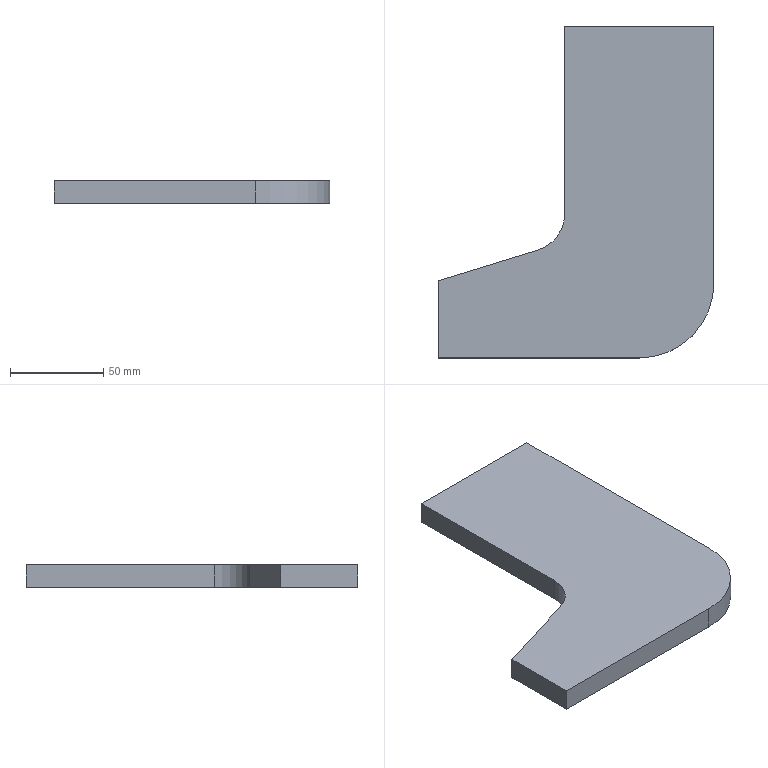Part | STEP file | Discharge manipulator bracket.SLDASM-2 | 1 solid | 10 faces | box 147.814 x 177.869 x 12 mm | volume 209292 mm3 | plane 8 | cylinder 2 | commonest cylinder face diameters 40 x1 80 x1
STEP:
#1=CARTESIAN_POINT('',(171.087,56.361,0.));
#2=VERTEX_POINT('',#1);
#3=CARTESIAN_POINT('',(171.087,15.,0.));
#4=VERTEX_POINT('',#3);
#5=CARTESIAN_POINT('',(171.087,15.,0.));
#6=DIRECTION('',(0.,-1.,0.));
#7=VECTOR('',#6,1000.);
#8=LINE('',#5,#7);
#9=EDGE_CURVE('',#2,#4,#8,.T.);
#10=ORIENTED_EDGE('',*,*,#9,.F.);
#11=CARTESIAN_POINT('',(171.087,56.361,-12.));
#12=VERTEX_POINT('',#11);
#13=CARTESIAN_POINT('',(171.087,56.361,-12.));
#14=DIRECTION('',(0.,0.,1.));
#15=VECTOR('',#14,1000.);
#16=LINE('',#13,#15);
#17=EDGE_CURVE('',#12,#2,#16,.T.);
#18=ORIENTED_EDGE('',*,*,#17,.F.);
#19=CARTESIAN_POINT('',(171.087,15.,-12.));
#20=VERTEX_POINT('',#19);
#21=CARTESIAN_POINT('',(171.087,15.,-12.));
#22=DIRECTION('',(0.,-1.,0.));
#23=VECTOR('',#22,1000.);
#24=LINE('',#21,#23);
#25=EDGE_CURVE('',#12,#20,#24,.T.);
#26=ORIENTED_EDGE('',*,*,#25,.T.);
#27=CARTESIAN_POINT('',(171.087,15.,-12.));
#28=DIRECTION('',(0.,0.,1.));
#29=VECTOR('',#28,1000.);
#30=LINE('',#27,#29);
#31=EDGE_CURVE('',#20,#4,#30,.T.);
#32=ORIENTED_EDGE('',*,*,#31,.T.);
#33=EDGE_LOOP('',(#10,#18,#26,#32));
#34=FACE_OUTER_BOUND('',#33,.T.);
#35=CARTESIAN_POINT('',(171.087,15.,-12.));
#36=DIRECTION('',(-1.,0.,0.));
#37=DIRECTION('',(0.,0.,1.));
#38=AXIS2_PLACEMENT_3D('',#35,#36,#37);
#39=PLANE('',#38);
#40=ADVANCED_FACE('',(#34),#39,.T.);
#41=CARTESIAN_POINT('',(224.795,72.924,0.));
#42=VERTEX_POINT('',#41);
#43=CARTESIAN_POINT('',(171.087,56.361,0.));
#44=DIRECTION('',(-0.9556,-0.2947,0.));
#45=VECTOR('',#44,1000.);
#46=LINE('',#43,#45);
#47=EDGE_CURVE('',#42,#2,#46,.T.);
#48=ORIENTED_EDGE('',*,*,#47,.F.);
#49=CARTESIAN_POINT('',(224.795,72.924,-12.));
#50=VERTEX_POINT('',#49);
#51=CARTESIAN_POINT('',(224.795,72.924,-12.));
#52=DIRECTION('',(0.,0.,-1.));
#53=VECTOR('',#52,1000.);
#54=LINE('',#51,#53);
#55=EDGE_CURVE('',#42,#50,#54,.T.);
#56=ORIENTED_EDGE('',*,*,#55,.T.);
#57=CARTESIAN_POINT('',(171.087,56.361,-12.));
#58=DIRECTION('',(-0.9556,-0.2947,0.));
#59=VECTOR('',#58,1000.);
#60=LINE('',#57,#59);
#61=EDGE_CURVE('',#50,#12,#60,.T.);
#62=ORIENTED_EDGE('',*,*,#61,.T.);
#63=ORIENTED_EDGE('',*,*,#17,.T.);
#64=EDGE_LOOP('',(#48,#56,#62,#63));
#65=FACE_OUTER_BOUND('',#64,.T.);
#66=CARTESIAN_POINT('',(171.087,56.361,-12.));
#67=DIRECTION('',(-0.2947,0.9556,0.));
#68=DIRECTION('',(-0.9556,-0.2947,0.));
#69=AXIS2_PLACEMENT_3D('',#66,#67,#68);
#70=PLANE('',#69);
#71=ADVANCED_FACE('',(#65),#70,.T.);
#72=CARTESIAN_POINT('',(238.901,192.869,-12.));
#73=VERTEX_POINT('',#72);
#74=CARTESIAN_POINT('',(238.901,92.035,-12.));
#75=VERTEX_POINT('',#74);
#76=CARTESIAN_POINT('',(238.901,77.274,-12.));
#77=DIRECTION('',(0.,-1.,0.));
#78=VECTOR('',#77,1000.);
#79=LINE('',#76,#78);
#80=EDGE_CURVE('',#73,#75,#79,.T.);
#81=ORIENTED_EDGE('',*,*,#80,.T.);
#82=CARTESIAN_POINT('',(238.901,92.035,0.));
#83=VERTEX_POINT('',#82);
#84=CARTESIAN_POINT('',(238.901,92.035,0.));
#85=DIRECTION('',(0.,0.,1.));
#86=VECTOR('',#85,1000.);
#87=LINE('',#84,#86);
#88=EDGE_CURVE('',#75,#83,#87,.T.);
#89=ORIENTED_EDGE('',*,*,#88,.T.);
#90=CARTESIAN_POINT('',(238.901,192.869,0.));
#91=VERTEX_POINT('',#90);
#92=CARTESIAN_POINT('',(238.901,77.274,0.));
#93=DIRECTION('',(0.,-1.,0.));
#94=VECTOR('',#93,1000.);
#95=LINE('',#92,#94);
#96=EDGE_CURVE('',#91,#83,#95,.T.);
#97=ORIENTED_EDGE('',*,*,#96,.F.);
#98=CARTESIAN_POINT('',(238.901,192.869,-12.));
#99=DIRECTION('',(0.,0.,1.));
#100=VECTOR('',#99,1000.);
#101=LINE('',#98,#100);
#102=EDGE_CURVE('',#73,#91,#101,.T.);
#103=ORIENTED_EDGE('',*,*,#102,.F.);
#104=EDGE_LOOP('',(#81,#89,#97,#103));
#105=FACE_OUTER_BOUND('',#104,.T.);
#106=CARTESIAN_POINT('',(238.901,77.274,-12.));
#107=DIRECTION('',(-1.,0.,0.));
#108=DIRECTION('',(0.,0.,1.));
#109=AXIS2_PLACEMENT_3D('',#106,#107,#108);
#110=PLANE('',#109);
#111=ADVANCED_FACE('',(#105),#110,.T.);
#112=CARTESIAN_POINT('',(318.901,192.869,0.));
#113=VERTEX_POINT('',#112);
#114=CARTESIAN_POINT('',(238.901,192.869,0.));
#115=DIRECTION('',(-1.,0.,0.));
#116=VECTOR('',#115,1000.);
#117=LINE('',#114,#116);
#118=EDGE_CURVE('',#113,#91,#117,.T.);
#119=ORIENTED_EDGE('',*,*,#118,.F.);
#120=CARTESIAN_POINT('',(318.901,192.869,-12.));
#121=VERTEX_POINT('',#120);
#122=CARTESIAN_POINT('',(318.901,192.869,-12.));
#123=DIRECTION('',(0.,0.,1.));
#124=VECTOR('',#123,1000.);
#125=LINE('',#122,#124);
#126=EDGE_CURVE('',#121,#113,#125,.T.);
#127=ORIENTED_EDGE('',*,*,#126,.F.);
#128=CARTESIAN_POINT('',(238.901,192.869,-12.));
#129=DIRECTION('',(-1.,0.,0.));
#130=VECTOR('',#129,1000.);
#131=LINE('',#128,#130);
#132=EDGE_CURVE('',#121,#73,#131,.T.);
#133=ORIENTED_EDGE('',*,*,#132,.T.);
#134=ORIENTED_EDGE('',*,*,#102,.T.);
#135=EDGE_LOOP('',(#119,#127,#133,#134));
#136=FACE_OUTER_BOUND('',#135,.T.);
#137=CARTESIAN_POINT('',(238.901,192.869,-12.));
#138=DIRECTION('',(0.,1.,0.));
#139=DIRECTION('',(-1.,0.,0.));
#140=AXIS2_PLACEMENT_3D('',#137,#138,#139);
#141=PLANE('',#140);
#142=ADVANCED_FACE('',(#136),#141,.T.);
#143=CARTESIAN_POINT('',(318.901,55.,0.));
#144=VERTEX_POINT('',#143);
#145=CARTESIAN_POINT('',(318.901,15.,0.));
#146=DIRECTION('',(0.,1.,0.));
#147=VECTOR('',#146,1000.);
#148=LINE('',#145,#147);
#149=EDGE_CURVE('',#144,#113,#148,.T.);
#150=ORIENTED_EDGE('',*,*,#149,.F.);
#151=CARTESIAN_POINT('',(318.901,55.,-12.));
#152=VERTEX_POINT('',#151);
#153=CARTESIAN_POINT('',(318.901,55.,-12.));
#154=DIRECTION('',(0.,0.,-1.));
#155=VECTOR('',#154,1000.);
#156=LINE('',#153,#155);
#157=EDGE_CURVE('',#144,#152,#156,.T.);
#158=ORIENTED_EDGE('',*,*,#157,.T.);
#159=CARTESIAN_POINT('',(318.901,15.,-12.));
#160=DIRECTION('',(0.,1.,0.));
#161=VECTOR('',#160,1000.);
#162=LINE('',#159,#161);
#163=EDGE_CURVE('',#152,#121,#162,.T.);
#164=ORIENTED_EDGE('',*,*,#163,.T.);
#165=ORIENTED_EDGE('',*,*,#126,.T.);
#166=EDGE_LOOP('',(#150,#158,#164,#165));
#167=FACE_OUTER_BOUND('',#166,.T.);
#168=CARTESIAN_POINT('',(318.901,15.,-12.));
#169=DIRECTION('',(1.,0.,0.));
#170=DIRECTION('',(0.,0.,-1.));
#171=AXIS2_PLACEMENT_3D('',#168,#169,#170);
#172=PLANE('',#171);
#173=ADVANCED_FACE('',(#167),#172,.T.);
#174=CARTESIAN_POINT('',(278.901,15.,-12.));
#175=VERTEX_POINT('',#174);
#176=CARTESIAN_POINT('',(171.087,15.,-12.));
#177=DIRECTION('',(1.,0.,0.));
#178=VECTOR('',#177,1000.);
#179=LINE('',#176,#178);
#180=EDGE_CURVE('',#20,#175,#179,.T.);
#181=ORIENTED_EDGE('',*,*,#180,.T.);
#182=CARTESIAN_POINT('',(278.901,15.,0.));
#183=VERTEX_POINT('',#182);
#184=CARTESIAN_POINT('',(278.901,15.,-12.));
#185=DIRECTION('',(0.,0.,1.));
#186=VECTOR('',#185,1000.);
#187=LINE('',#184,#186);
#188=EDGE_CURVE('',#175,#183,#187,.T.);
#189=ORIENTED_EDGE('',*,*,#188,.T.);
#190=CARTESIAN_POINT('',(171.087,15.,0.));
#191=DIRECTION('',(1.,0.,0.));
#192=VECTOR('',#191,1000.);
#193=LINE('',#190,#192);
#194=EDGE_CURVE('',#4,#183,#193,.T.);
#195=ORIENTED_EDGE('',*,*,#194,.F.);
#196=ORIENTED_EDGE('',*,*,#31,.F.);
#197=EDGE_LOOP('',(#181,#189,#195,#196));
#198=FACE_OUTER_BOUND('',#197,.T.);
#199=CARTESIAN_POINT('',(171.087,15.,-12.));
#200=DIRECTION('',(0.,-1.,0.));
#201=DIRECTION('',(0.,0.,-1.));
#202=AXIS2_PLACEMENT_3D('',#199,#200,#201);
#203=PLANE('',#202);
#204=ADVANCED_FACE('',(#198),#203,.T.);
#205=ORIENTED_EDGE('',*,*,#163,.F.);
#206=CARTESIAN_POINT('',(278.901,55.,-12.));
#207=DIRECTION('',(0.,0.,-1.));
#208=DIRECTION('',(-1.,0.,0.));
#209=AXIS2_PLACEMENT_3D('',#206,#207,#208);
#210=CIRCLE('',#209,40.);
#211=EDGE_CURVE('',#152,#175,#210,.T.);
#212=ORIENTED_EDGE('',*,*,#211,.T.);
#213=ORIENTED_EDGE('',*,*,#180,.F.);
#214=ORIENTED_EDGE('',*,*,#25,.F.);
#215=ORIENTED_EDGE('',*,*,#61,.F.);
#216=CARTESIAN_POINT('',(218.901,92.035,-12.));
#217=DIRECTION('',(0.,0.,1.));
#218=DIRECTION('',(-1.,0.,0.));
#219=AXIS2_PLACEMENT_3D('',#216,#217,#218);
#220=CIRCLE('',#219,20.);
#221=EDGE_CURVE('',#50,#75,#220,.T.);
#222=ORIENTED_EDGE('',*,*,#221,.T.);
#223=ORIENTED_EDGE('',*,*,#80,.F.);
#224=ORIENTED_EDGE('',*,*,#132,.F.);
#225=EDGE_LOOP('',(#205,#212,#213,#214,#215,#222,#223,#224));
#226=FACE_OUTER_BOUND('',#225,.T.);
#227=CARTESIAN_POINT('',(171.087,192.869,-12.));
#228=DIRECTION('',(0.,0.,-1.));
#229=DIRECTION('',(-1.,0.,0.));
#230=AXIS2_PLACEMENT_3D('',#227,#228,#229);
#231=PLANE('',#230);
#232=ADVANCED_FACE('',(#226),#231,.T.);
#233=ORIENTED_EDGE('',*,*,#194,.T.);
#234=CARTESIAN_POINT('',(278.901,55.,0.));
#235=DIRECTION('',(0.,0.,1.));
#236=DIRECTION('',(-1.,0.,0.));
#237=AXIS2_PLACEMENT_3D('',#234,#235,#236);
#238=CIRCLE('',#237,40.);
#239=EDGE_CURVE('',#183,#144,#238,.T.);
#240=ORIENTED_EDGE('',*,*,#239,.T.);
#241=ORIENTED_EDGE('',*,*,#149,.T.);
#242=ORIENTED_EDGE('',*,*,#118,.T.);
#243=ORIENTED_EDGE('',*,*,#96,.T.);
#244=CARTESIAN_POINT('',(218.901,92.035,0.));
#245=DIRECTION('',(0.,0.,-1.));
#246=DIRECTION('',(-1.,0.,0.));
#247=AXIS2_PLACEMENT_3D('',#244,#245,#246);
#248=CIRCLE('',#247,20.);
#249=EDGE_CURVE('',#83,#42,#248,.T.);
#250=ORIENTED_EDGE('',*,*,#249,.T.);
#251=ORIENTED_EDGE('',*,*,#47,.T.);
#252=ORIENTED_EDGE('',*,*,#9,.T.);
#253=EDGE_LOOP('',(#233,#240,#241,#242,#243,#250,#251,#252));
#254=FACE_OUTER_BOUND('',#253,.T.);
#255=CARTESIAN_POINT('',(171.087,192.869,0.));
#256=DIRECTION('',(0.,0.,-1.));
#257=DIRECTION('',(-1.,0.,0.));
#258=AXIS2_PLACEMENT_3D('',#255,#256,#257);
#259=PLANE('',#258);
#260=ADVANCED_FACE('',(#254),#259,.F.);
#261=ORIENTED_EDGE('',*,*,#221,.F.);
#262=ORIENTED_EDGE('',*,*,#55,.F.);
#263=ORIENTED_EDGE('',*,*,#249,.F.);
#264=ORIENTED_EDGE('',*,*,#88,.F.);
#265=EDGE_LOOP('',(#261,#262,#263,#264));
#266=FACE_OUTER_BOUND('',#265,.T.);
#267=CARTESIAN_POINT('',(218.901,92.035,-12.));
#268=DIRECTION('',(0.,0.,-1.));
#269=DIRECTION('',(-1.,0.,0.));
#270=AXIS2_PLACEMENT_3D('',#267,#268,#269);
#271=CYLINDRICAL_SURFACE('',#270,20.);
#272=ADVANCED_FACE('',(#266),#271,.F.);
#273=ORIENTED_EDGE('',*,*,#211,.F.);
#274=ORIENTED_EDGE('',*,*,#157,.F.);
#275=ORIENTED_EDGE('',*,*,#239,.F.);
#276=ORIENTED_EDGE('',*,*,#188,.F.);
#277=EDGE_LOOP('',(#273,#274,#275,#276));
#278=FACE_OUTER_BOUND('',#277,.T.);
#279=CARTESIAN_POINT('',(278.901,55.,-12.));
#280=DIRECTION('',(0.,0.,1.));
#281=DIRECTION('',(1.,0.,0.));
#282=AXIS2_PLACEMENT_3D('',#279,#280,#281);
#283=CYLINDRICAL_SURFACE('',#282,40.);
#284=ADVANCED_FACE('',(#278),#283,.T.);
#285=CLOSED_SHELL('',(#40,#71,#111,#142,#173,#204,#232,#260,#272,#284));
#286=MANIFOLD_SOLID_BREP('',#285);
#287=CARTESIAN_POINT('',(0.,0.,0.));
#288=DIRECTION('',(0.,0.,1.));
#289=DIRECTION('',(1.,0.,0.));
#290=AXIS2_PLACEMENT_3D('',#287,#288,#289);
#291=(LENGTH_UNIT()NAMED_UNIT(*)SI_UNIT(.MILLI.,.METRE.));
#292=UNCERTAINTY_MEASURE_WITH_UNIT(LENGTH_MEASURE(0.00001),#291,'','');
#293=(NAMED_UNIT(*)PLANE_ANGLE_UNIT()SI_UNIT($,.RADIAN.));
#294=(NAMED_UNIT(*)SI_UNIT($,.STERADIAN.)SOLID_ANGLE_UNIT());
#295=(GEOMETRIC_REPRESENTATION_CONTEXT(3)GLOBAL_UNCERTAINTY_ASSIGNED_CONTEXT((#292))GLOBAL_UNIT_ASSIGNED_CONTEXT((#291,#293,#294))REPRESENTATION_CONTEXT('',''));
#296=ADVANCED_BREP_SHAPE_REPRESENTATION('',(#286,#290),#295);